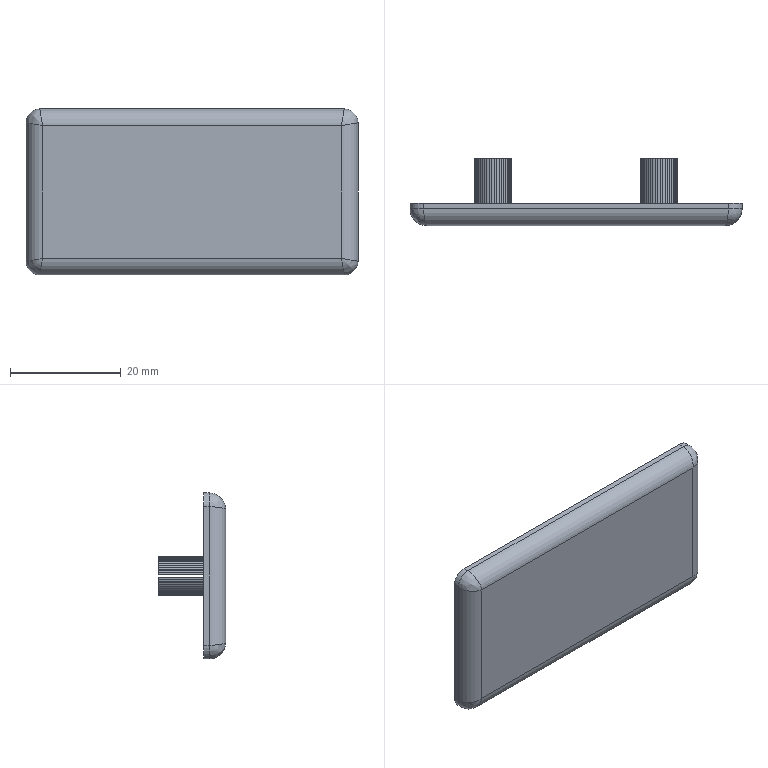Part | STEP file | 1 solid | 227 faces | box 60 x 12.2 x 30 mm | volume 5483 mm3 | cylinder 112 | plane 111 | spline 4 | commonest cylinder face diameters 6.6 x48 7 x46 5 x8 4.9 x6 6 x4